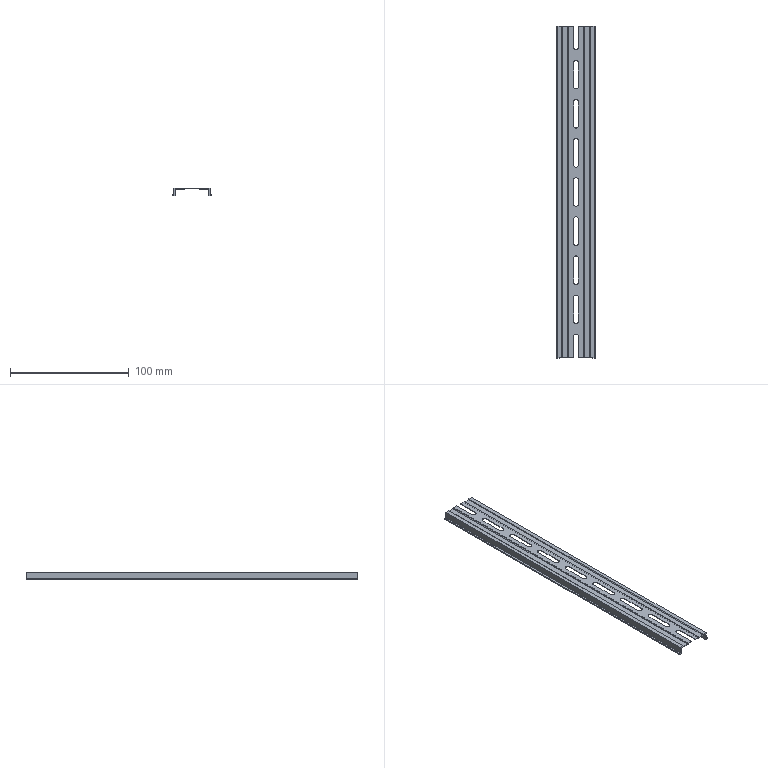Part | STEP file | Mounting plate 2 | 1 solid | 62 faces | box 33.46 x 280 x 6.5 mm | volume 8894 mm3 | plane 40 | cylinder 22 | commonest cylinder face diameters 4.2 x16 1 x6